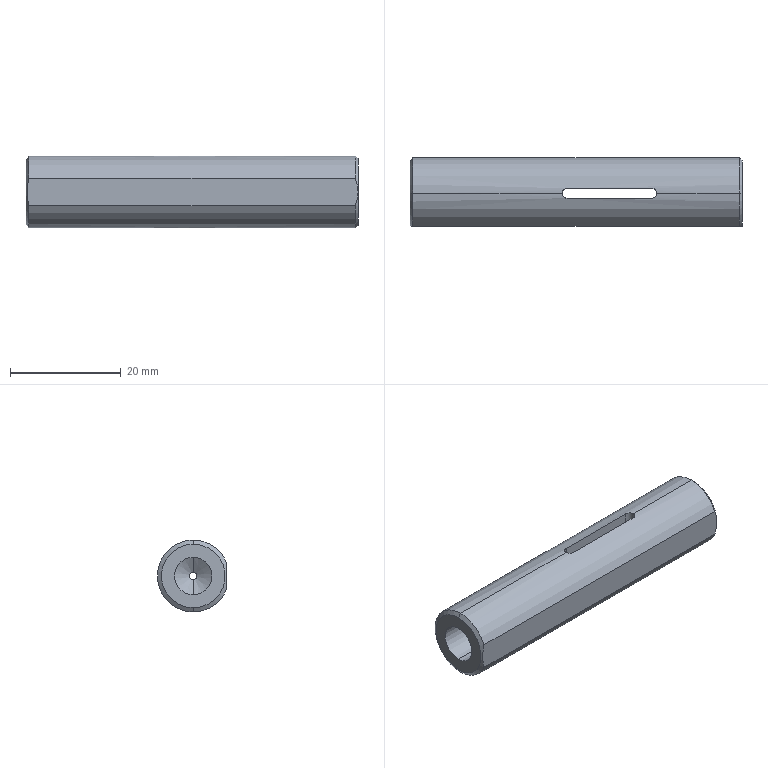Part | STEP file | detection slide rod | 1 solid | 27 faces | box 60 x 12.5 x 13 mm | volume 5988 mm3 | cylinder 13 | cone 7 | plane 7 | commonest cylinder face diameters 1.8 x6 13 x3 1.3 x2 6.8 x2